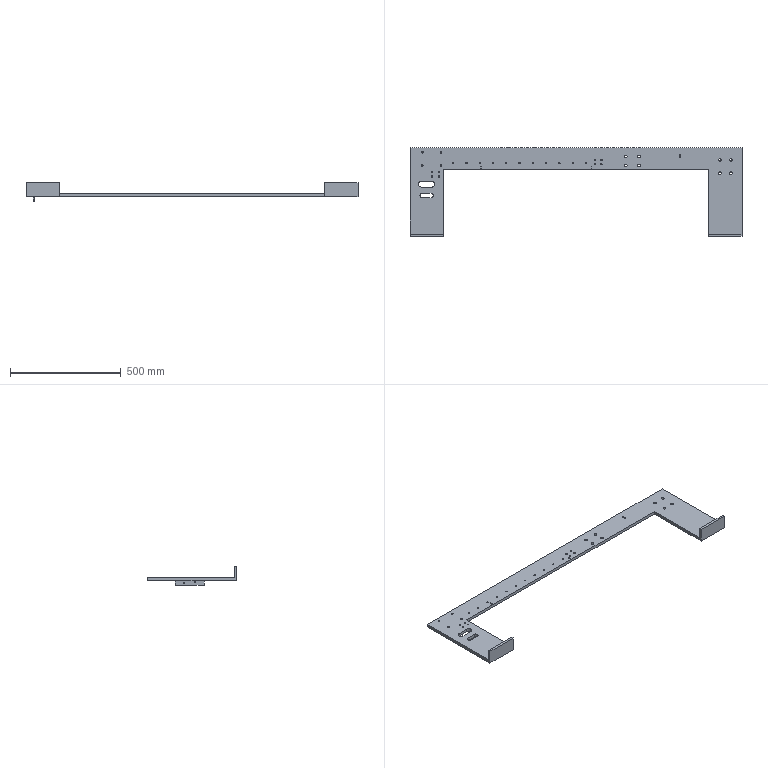Part | STEP file | Middle plate 1 | 1 solid | 108 faces | box 1500 x 400 x 84 mm | volume 3461326 mm3 | cylinder 84 | plane 24 | commonest cylinder face diameters 6 x40 12 x16 4 x14 8 x8 20 x3 25 x3